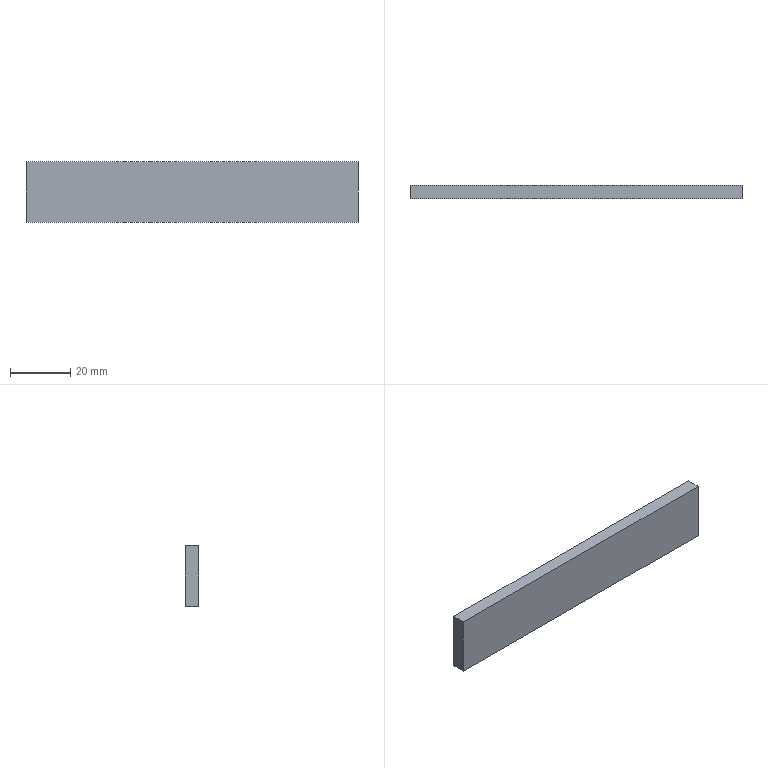Part | STEP file | Guide wheel mechanism revised.sldasm-Part-57 | 1 solid | 6 faces | box 110 x 4.5 x 20 mm | volume 9900 mm3 | plane 6
STEP:
#1=CARTESIAN_POINT('',(368.,29.5,-10.));
#2=VERTEX_POINT('',#1);
#3=CARTESIAN_POINT('',(258.,29.5,-10.));
#4=VERTEX_POINT('',#3);
#5=CARTESIAN_POINT('',(1300.,29.5,-10.));
#6=DIRECTION('',(-1.,0.,0.));
#7=VECTOR('',#6,1000.);
#8=LINE('',#5,#7);
#9=EDGE_CURVE('',#2,#4,#8,.T.);
#10=ORIENTED_EDGE('',*,*,#9,.F.);
#11=CARTESIAN_POINT('',(368.,25.,-10.));
#12=VERTEX_POINT('',#11);
#13=CARTESIAN_POINT('',(368.,0.,-10.));
#14=DIRECTION('',(0.,-1.,0.));
#15=VECTOR('',#14,1000.);
#16=LINE('',#13,#15);
#17=EDGE_CURVE('',#2,#12,#16,.T.);
#18=ORIENTED_EDGE('',*,*,#17,.T.);
#19=CARTESIAN_POINT('',(258.,25.,-10.));
#20=VERTEX_POINT('',#19);
#21=CARTESIAN_POINT('',(1300.,25.,-10.));
#22=DIRECTION('',(-1.,0.,0.));
#23=VECTOR('',#22,1000.);
#24=LINE('',#21,#23);
#25=EDGE_CURVE('',#12,#20,#24,.T.);
#26=ORIENTED_EDGE('',*,*,#25,.T.);
#27=CARTESIAN_POINT('',(258.,0.,-10.));
#28=DIRECTION('',(0.,1.,0.));
#29=VECTOR('',#28,1000.);
#30=LINE('',#27,#29);
#31=EDGE_CURVE('',#20,#4,#30,.T.);
#32=ORIENTED_EDGE('',*,*,#31,.T.);
#33=EDGE_LOOP('',(#10,#18,#26,#32));
#34=FACE_OUTER_BOUND('',#33,.T.);
#35=CARTESIAN_POINT('',(0.,0.,-10.));
#36=DIRECTION('',(0.,0.,1.));
#37=DIRECTION('',(1.,0.,0.));
#38=AXIS2_PLACEMENT_3D('',#35,#36,#37);
#39=PLANE('',#38);
#40=ADVANCED_FACE('',(#34),#39,.F.);
#41=CARTESIAN_POINT('',(368.,25.,10.));
#42=VERTEX_POINT('',#41);
#43=CARTESIAN_POINT('',(368.,25.,10.));
#44=DIRECTION('',(0.,0.,-1.));
#45=VECTOR('',#44,1000.);
#46=LINE('',#43,#45);
#47=EDGE_CURVE('',#42,#12,#46,.T.);
#48=ORIENTED_EDGE('',*,*,#47,.F.);
#49=CARTESIAN_POINT('',(258.,25.,10.));
#50=VERTEX_POINT('',#49);
#51=CARTESIAN_POINT('',(1300.,25.,10.));
#52=DIRECTION('',(-1.,0.,0.));
#53=VECTOR('',#52,1000.);
#54=LINE('',#51,#53);
#55=EDGE_CURVE('',#42,#50,#54,.T.);
#56=ORIENTED_EDGE('',*,*,#55,.T.);
#57=CARTESIAN_POINT('',(258.,25.,10.));
#58=DIRECTION('',(0.,0.,1.));
#59=VECTOR('',#58,1000.);
#60=LINE('',#57,#59);
#61=EDGE_CURVE('',#20,#50,#60,.T.);
#62=ORIENTED_EDGE('',*,*,#61,.F.);
#63=ORIENTED_EDGE('',*,*,#25,.F.);
#64=EDGE_LOOP('',(#48,#56,#62,#63));
#65=FACE_OUTER_BOUND('',#64,.T.);
#66=CARTESIAN_POINT('',(1300.,25.,10.));
#67=DIRECTION('',(0.,-1.,0.));
#68=DIRECTION('',(0.,0.,-1.));
#69=AXIS2_PLACEMENT_3D('',#66,#67,#68);
#70=PLANE('',#69);
#71=ADVANCED_FACE('',(#65),#70,.T.);
#72=CARTESIAN_POINT('',(368.,29.5,10.));
#73=VERTEX_POINT('',#72);
#74=CARTESIAN_POINT('',(258.,29.5,10.));
#75=VERTEX_POINT('',#74);
#76=CARTESIAN_POINT('',(1300.,29.5,10.));
#77=DIRECTION('',(-1.,0.,0.));
#78=VECTOR('',#77,1000.);
#79=LINE('',#76,#78);
#80=EDGE_CURVE('',#73,#75,#79,.T.);
#81=ORIENTED_EDGE('',*,*,#80,.F.);
#82=CARTESIAN_POINT('',(368.,29.5,-15.));
#83=DIRECTION('',(0.,0.,1.));
#84=VECTOR('',#83,1000.);
#85=LINE('',#82,#84);
#86=EDGE_CURVE('',#2,#73,#85,.T.);
#87=ORIENTED_EDGE('',*,*,#86,.F.);
#88=ORIENTED_EDGE('',*,*,#9,.T.);
#89=CARTESIAN_POINT('',(258.,29.5,-15.));
#90=DIRECTION('',(0.,0.,-1.));
#91=VECTOR('',#90,1000.);
#92=LINE('',#89,#91);
#93=EDGE_CURVE('',#75,#4,#92,.T.);
#94=ORIENTED_EDGE('',*,*,#93,.F.);
#95=EDGE_LOOP('',(#81,#87,#88,#94));
#96=FACE_OUTER_BOUND('',#95,.T.);
#97=CARTESIAN_POINT('',(1300.,29.5,10.));
#98=DIRECTION('',(0.,-1.,0.));
#99=DIRECTION('',(0.,0.,-1.));
#100=AXIS2_PLACEMENT_3D('',#97,#98,#99);
#101=PLANE('',#100);
#102=ADVANCED_FACE('',(#96),#101,.F.);
#103=CARTESIAN_POINT('',(368.,0.,10.));
#104=DIRECTION('',(0.,-1.,0.));
#105=VECTOR('',#104,1000.);
#106=LINE('',#103,#105);
#107=EDGE_CURVE('',#73,#42,#106,.T.);
#108=ORIENTED_EDGE('',*,*,#107,.F.);
#109=ORIENTED_EDGE('',*,*,#80,.T.);
#110=CARTESIAN_POINT('',(258.,0.,10.));
#111=DIRECTION('',(0.,1.,0.));
#112=VECTOR('',#111,1000.);
#113=LINE('',#110,#112);
#114=EDGE_CURVE('',#50,#75,#113,.T.);
#115=ORIENTED_EDGE('',*,*,#114,.F.);
#116=ORIENTED_EDGE('',*,*,#55,.F.);
#117=EDGE_LOOP('',(#108,#109,#115,#116));
#118=FACE_OUTER_BOUND('',#117,.T.);
#119=CARTESIAN_POINT('',(0.,0.,10.));
#120=DIRECTION('',(0.,0.,1.));
#121=DIRECTION('',(1.,0.,0.));
#122=AXIS2_PLACEMENT_3D('',#119,#120,#121);
#123=PLANE('',#122);
#124=ADVANCED_FACE('',(#118),#123,.T.);
#125=ORIENTED_EDGE('',*,*,#114,.T.);
#126=ORIENTED_EDGE('',*,*,#93,.T.);
#127=ORIENTED_EDGE('',*,*,#31,.F.);
#128=ORIENTED_EDGE('',*,*,#61,.T.);
#129=EDGE_LOOP('',(#125,#126,#127,#128));
#130=FACE_OUTER_BOUND('',#129,.T.);
#131=CARTESIAN_POINT('',(258.,-30.5,-15.));
#132=DIRECTION('',(1.,0.,0.));
#133=DIRECTION('',(0.,0.,-1.));
#134=AXIS2_PLACEMENT_3D('',#131,#132,#133);
#135=PLANE('',#134);
#136=ADVANCED_FACE('',(#130),#135,.F.);
#137=ORIENTED_EDGE('',*,*,#86,.T.);
#138=ORIENTED_EDGE('',*,*,#107,.T.);
#139=ORIENTED_EDGE('',*,*,#47,.T.);
#140=ORIENTED_EDGE('',*,*,#17,.F.);
#141=EDGE_LOOP('',(#137,#138,#139,#140));
#142=FACE_OUTER_BOUND('',#141,.T.);
#143=CARTESIAN_POINT('',(368.,-30.5,-15.));
#144=DIRECTION('',(-1.,0.,0.));
#145=DIRECTION('',(0.,0.,1.));
#146=AXIS2_PLACEMENT_3D('',#143,#144,#145);
#147=PLANE('',#146);
#148=ADVANCED_FACE('',(#142),#147,.F.);
#149=CLOSED_SHELL('',(#40,#71,#102,#124,#136,#148));
#150=MANIFOLD_SOLID_BREP('',#149);
#151=CARTESIAN_POINT('',(0.,0.,0.));
#152=DIRECTION('',(0.,0.,1.));
#153=DIRECTION('',(1.,0.,0.));
#154=AXIS2_PLACEMENT_3D('',#151,#152,#153);
#155=(LENGTH_UNIT()NAMED_UNIT(*)SI_UNIT(.MILLI.,.METRE.));
#156=UNCERTAINTY_MEASURE_WITH_UNIT(LENGTH_MEASURE(0.00001),#155,'','');
#157=(NAMED_UNIT(*)PLANE_ANGLE_UNIT()SI_UNIT($,.RADIAN.));
#158=(NAMED_UNIT(*)SI_UNIT($,.STERADIAN.)SOLID_ANGLE_UNIT());
#159=(GEOMETRIC_REPRESENTATION_CONTEXT(3)GLOBAL_UNCERTAINTY_ASSIGNED_CONTEXT((#156))GLOBAL_UNIT_ASSIGNED_CONTEXT((#155,#157,#158))REPRESENTATION_CONTEXT('',''));
#160=ADVANCED_BREP_SHAPE_REPRESENTATION('',(#150,#154),#159);